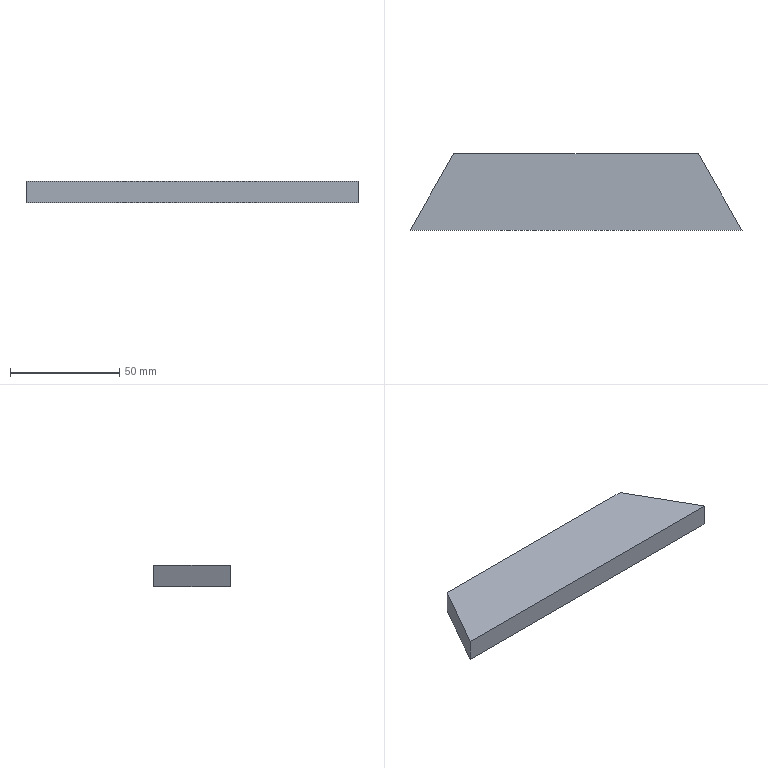Part | SolidWorks | features Extrusion 1 | 1 solid | 6 faces | box 152 x 35 x 10 mm | volume 46200 mm3 | plane 6
STEP:
#1=CARTESIAN_POINT('',(20.,35.,0.));
#2=VERTEX_POINT('',#1);
#3=CARTESIAN_POINT('',(0.,0.,0.));
#4=VERTEX_POINT('',#3);
#5=CARTESIAN_POINT('',(20.,35.,0.));
#6=DIRECTION('',(-0.4961,-0.8682,0.));
#7=VECTOR('',#6,1000.);
#8=LINE('',#5,#7);
#9=EDGE_CURVE('',#2,#4,#8,.T.);
#10=ORIENTED_EDGE('',*,*,#9,.T.);
#11=CARTESIAN_POINT('',(0.,0.,10.));
#12=VERTEX_POINT('',#11);
#13=CARTESIAN_POINT('',(0.,0.,10.));
#14=DIRECTION('',(0.,0.,-1.));
#15=VECTOR('',#14,1000.);
#16=LINE('',#13,#15);
#17=EDGE_CURVE('',#12,#4,#16,.T.);
#18=ORIENTED_EDGE('',*,*,#17,.F.);
#19=CARTESIAN_POINT('',(20.,35.,10.));
#20=VERTEX_POINT('',#19);
#21=CARTESIAN_POINT('',(20.,35.,10.));
#22=DIRECTION('',(-0.4961,-0.8682,0.));
#23=VECTOR('',#22,1000.);
#24=LINE('',#21,#23);
#25=EDGE_CURVE('',#20,#12,#24,.T.);
#26=ORIENTED_EDGE('',*,*,#25,.F.);
#27=CARTESIAN_POINT('',(20.,35.,10.));
#28=DIRECTION('',(0.,0.,-1.));
#29=VECTOR('',#28,1000.);
#30=LINE('',#27,#29);
#31=EDGE_CURVE('',#20,#2,#30,.T.);
#32=ORIENTED_EDGE('',*,*,#31,.T.);
#33=EDGE_LOOP('',(#10,#18,#26,#32));
#34=FACE_OUTER_BOUND('',#33,.T.);
#35=CARTESIAN_POINT('',(20.,35.,10.));
#36=DIRECTION('',(0.8682,-0.4961,0.));
#37=DIRECTION('',(0.4961,0.8682,0.));
#38=AXIS2_PLACEMENT_3D('',#35,#36,#37);
#39=PLANE('',#38);
#40=ADVANCED_FACE('',(#34),#39,.F.);
#41=CARTESIAN_POINT('',(152.,0.,0.));
#42=VERTEX_POINT('',#41);
#43=CARTESIAN_POINT('',(0.,0.,0.));
#44=DIRECTION('',(1.,0.,0.));
#45=VECTOR('',#44,1000.);
#46=LINE('',#43,#45);
#47=EDGE_CURVE('',#4,#42,#46,.T.);
#48=ORIENTED_EDGE('',*,*,#47,.T.);
#49=CARTESIAN_POINT('',(152.,0.,10.));
#50=VERTEX_POINT('',#49);
#51=CARTESIAN_POINT('',(152.,0.,10.));
#52=DIRECTION('',(0.,0.,-1.));
#53=VECTOR('',#52,1000.);
#54=LINE('',#51,#53);
#55=EDGE_CURVE('',#50,#42,#54,.T.);
#56=ORIENTED_EDGE('',*,*,#55,.F.);
#57=CARTESIAN_POINT('',(0.,0.,10.));
#58=DIRECTION('',(1.,0.,0.));
#59=VECTOR('',#58,1000.);
#60=LINE('',#57,#59);
#61=EDGE_CURVE('',#12,#50,#60,.T.);
#62=ORIENTED_EDGE('',*,*,#61,.F.);
#63=ORIENTED_EDGE('',*,*,#17,.T.);
#64=EDGE_LOOP('',(#48,#56,#62,#63));
#65=FACE_OUTER_BOUND('',#64,.T.);
#66=CARTESIAN_POINT('',(0.,0.,10.));
#67=DIRECTION('',(0.,1.,0.));
#68=DIRECTION('',(0.,0.,1.));
#69=AXIS2_PLACEMENT_3D('',#66,#67,#68);
#70=PLANE('',#69);
#71=ADVANCED_FACE('',(#65),#70,.F.);
#72=CARTESIAN_POINT('',(132.,35.,0.));
#73=VERTEX_POINT('',#72);
#74=CARTESIAN_POINT('',(152.,0.,0.));
#75=DIRECTION('',(-0.4961,0.8682,0.));
#76=VECTOR('',#75,1000.);
#77=LINE('',#74,#76);
#78=EDGE_CURVE('',#42,#73,#77,.T.);
#79=ORIENTED_EDGE('',*,*,#78,.T.);
#80=CARTESIAN_POINT('',(132.,35.,10.));
#81=VERTEX_POINT('',#80);
#82=CARTESIAN_POINT('',(132.,35.,10.));
#83=DIRECTION('',(0.,0.,-1.));
#84=VECTOR('',#83,1000.);
#85=LINE('',#82,#84);
#86=EDGE_CURVE('',#81,#73,#85,.T.);
#87=ORIENTED_EDGE('',*,*,#86,.F.);
#88=CARTESIAN_POINT('',(152.,0.,10.));
#89=DIRECTION('',(-0.4961,0.8682,0.));
#90=VECTOR('',#89,1000.);
#91=LINE('',#88,#90);
#92=EDGE_CURVE('',#50,#81,#91,.T.);
#93=ORIENTED_EDGE('',*,*,#92,.F.);
#94=ORIENTED_EDGE('',*,*,#55,.T.);
#95=EDGE_LOOP('',(#79,#87,#93,#94));
#96=FACE_OUTER_BOUND('',#95,.T.);
#97=CARTESIAN_POINT('',(152.,0.,10.));
#98=DIRECTION('',(-0.8682,-0.4961,0.));
#99=DIRECTION('',(0.4961,-0.8682,0.));
#100=AXIS2_PLACEMENT_3D('',#97,#98,#99);
#101=PLANE('',#100);
#102=ADVANCED_FACE('',(#96),#101,.F.);
#103=CARTESIAN_POINT('',(132.,35.,0.));
#104=DIRECTION('',(-1.,0.,0.));
#105=VECTOR('',#104,1000.);
#106=LINE('',#103,#105);
#107=EDGE_CURVE('',#73,#2,#106,.T.);
#108=ORIENTED_EDGE('',*,*,#107,.T.);
#109=ORIENTED_EDGE('',*,*,#31,.F.);
#110=CARTESIAN_POINT('',(132.,35.,10.));
#111=DIRECTION('',(-1.,0.,0.));
#112=VECTOR('',#111,1000.);
#113=LINE('',#110,#112);
#114=EDGE_CURVE('',#81,#20,#113,.T.);
#115=ORIENTED_EDGE('',*,*,#114,.F.);
#116=ORIENTED_EDGE('',*,*,#86,.T.);
#117=EDGE_LOOP('',(#108,#109,#115,#116));
#118=FACE_OUTER_BOUND('',#117,.T.);
#119=CARTESIAN_POINT('',(132.,35.,10.));
#120=DIRECTION('',(0.,-1.,0.));
#121=DIRECTION('',(0.,0.,-1.));
#122=AXIS2_PLACEMENT_3D('',#119,#120,#121);
#123=PLANE('',#122);
#124=ADVANCED_FACE('',(#118),#123,.F.);
#125=ORIENTED_EDGE('',*,*,#25,.T.);
#126=ORIENTED_EDGE('',*,*,#61,.T.);
#127=ORIENTED_EDGE('',*,*,#92,.T.);
#128=ORIENTED_EDGE('',*,*,#114,.T.);
#129=EDGE_LOOP('',(#125,#126,#127,#128));
#130=FACE_OUTER_BOUND('',#129,.T.);
#131=CARTESIAN_POINT('',(0.,0.,10.));
#132=DIRECTION('',(0.,0.,1.));
#133=DIRECTION('',(1.,0.,0.));
#134=AXIS2_PLACEMENT_3D('',#131,#132,#133);
#135=PLANE('',#134);
#136=ADVANCED_FACE('',(#130),#135,.T.);
#137=ORIENTED_EDGE('',*,*,#9,.F.);
#138=ORIENTED_EDGE('',*,*,#107,.F.);
#139=ORIENTED_EDGE('',*,*,#78,.F.);
#140=ORIENTED_EDGE('',*,*,#47,.F.);
#141=EDGE_LOOP('',(#137,#138,#139,#140));
#142=FACE_OUTER_BOUND('',#141,.T.);
#143=CARTESIAN_POINT('',(0.,0.,0.));
#144=DIRECTION('',(0.,0.,1.));
#145=DIRECTION('',(1.,0.,0.));
#146=AXIS2_PLACEMENT_3D('',#143,#144,#145);
#147=PLANE('',#146);
#148=ADVANCED_FACE('',(#142),#147,.F.);
#149=CLOSED_SHELL('',(#40,#71,#102,#124,#136,#148));
#150=MANIFOLD_SOLID_BREP('',#149);
#151=CARTESIAN_POINT('',(0.,0.,0.));
#152=DIRECTION('',(0.,0.,1.));
#153=DIRECTION('',(1.,0.,0.));
#154=AXIS2_PLACEMENT_3D('',#151,#152,#153);
#155=(LENGTH_UNIT()NAMED_UNIT(*)SI_UNIT(.MILLI.,.METRE.));
#156=UNCERTAINTY_MEASURE_WITH_UNIT(LENGTH_MEASURE(0.00001),#155,'','');
#157=(NAMED_UNIT(*)PLANE_ANGLE_UNIT()SI_UNIT($,.RADIAN.));
#158=(NAMED_UNIT(*)SI_UNIT($,.STERADIAN.)SOLID_ANGLE_UNIT());
#159=(GEOMETRIC_REPRESENTATION_CONTEXT(3)GLOBAL_UNCERTAINTY_ASSIGNED_CONTEXT((#156))GLOBAL_UNIT_ASSIGNED_CONTEXT((#155,#157,#158))REPRESENTATION_CONTEXT('',''));
#160=ADVANCED_BREP_SHAPE_REPRESENTATION('',(#150,#154),#159);